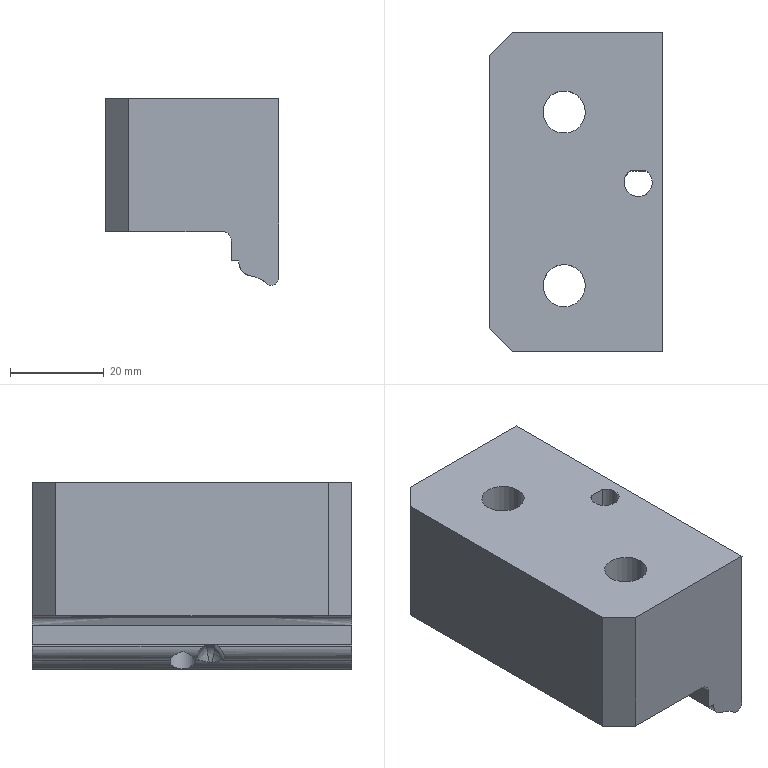Part | 1 solid | 34 faces | box 37.011 x 68 x 39.792 mm | volume 70310 mm3 | plane 16 | cylinder 14 | spline 3 | other 1 | commonest cylinder face diameters 9 x4 14 x4 6.4 x2 11.371 x2 3.1 x1 6 x1